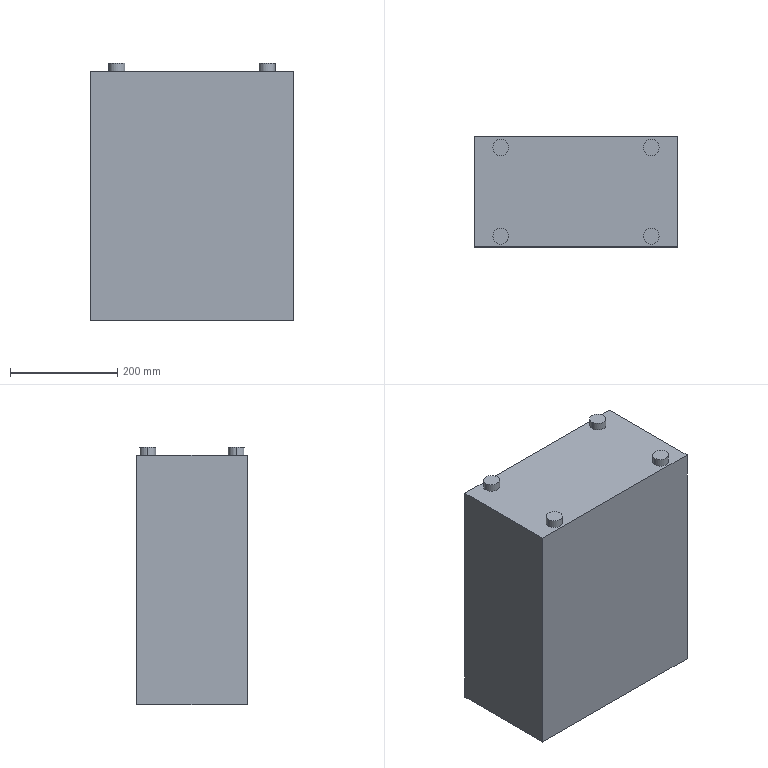Part | STEP file | PC | 1 solid | 18 faces | box 380 x 205 x 480 mm | volume 36265912 mm3 | plane 10 | cylinder 8 | commonest cylinder face diameters 30 x8
STEP:
#1=CARTESIAN_POINT('',(0.,0.,0.));
#2=DIRECTION('',(0.,0.,1.));
#3=DIRECTION('',(1.,0.,0.));
#4=AXIS2_PLACEMENT_3D('',#1,#2,#3);
#5=CARTESIAN_POINT('',(-125.,82.5,247.5));
#6=VERTEX_POINT('',#5);
#7=CARTESIAN_POINT('',(-155.,82.5,247.5));
#8=VERTEX_POINT('',#7);
#9=CARTESIAN_POINT('',(-140.,82.5,247.5));
#10=DIRECTION('',(0.,0.,1.));
#11=DIRECTION('',(-1.,0.,0.));
#12=AXIS2_PLACEMENT_3D('',#9,#10,#11);
#13=CIRCLE('',#12,15.);
#14=CARTESIAN_POINT('',(-140.,82.5,247.5));
#15=DIRECTION('',(0.,0.,-1.));
#16=DIRECTION('',(-1.,0.,0.));
#17=AXIS2_PLACEMENT_3D('',#14,#15,#16);
#18=CYLINDRICAL_SURFACE('',#17,15.);
#19=CARTESIAN_POINT('',(6.283,0.));
#20=DIRECTION('',(-1.,0.));
#21=VECTOR('',#20,1.);
#22=LINE('',#19,#21);
#23=(GEOMETRIC_REPRESENTATION_CONTEXT(2)PARAMETRIC_REPRESENTATION_CONTEXT()REPRESENTATION_CONTEXT('',''));
#24=DEFINITIONAL_REPRESENTATION('',(#22),#23);
#25=PCURVE('',#18,#24);
#26=CARTESIAN_POINT('',(-140.,82.5,247.5));
#27=DIRECTION('',(0.,0.,-1.));
#28=DIRECTION('',(-1.,0.,0.));
#29=AXIS2_PLACEMENT_3D('',#26,#27,#28);
#30=PLANE('',#29);
#31=CARTESIAN_POINT('',(15.,0.));
#32=CARTESIAN_POINT('',(15.,-25.981));
#33=CARTESIAN_POINT('',(-7.5,-12.99));
#34=CARTESIAN_POINT('',(-30.,0.));
#35=CARTESIAN_POINT('',(-7.5,12.99));
#36=CARTESIAN_POINT('',(15.,25.981));
#37=CARTESIAN_POINT('',(15.,0.));
#38=(BOUNDED_CURVE()B_SPLINE_CURVE(2,(#31,#32,#33,#34,#35,#36,#37),.UNSPECIFIED.,.T.,.F.)B_SPLINE_CURVE_WITH_KNOTS((1,2,2,2,2,1),(-2.094,0.,2.094,4.189,6.283,8.378),.UNSPECIFIED.)CURVE()GEOMETRIC_REPRESENTATION_ITEM()RATIONAL_B_SPLINE_CURVE((1.,0.5,1.,0.5,1.,0.5,1.))REPRESENTATION_ITEM(''));
#39=(GEOMETRIC_REPRESENTATION_CONTEXT(2)PARAMETRIC_REPRESENTATION_CONTEXT()REPRESENTATION_CONTEXT('',''));
#40=DEFINITIONAL_REPRESENTATION('',(#38),#39);
#41=PCURVE('',#30,#40);
#42=SURFACE_CURVE('',#13,(#25,#41),.PCURVE_S1.);
#43=EDGE_CURVE('',#6,#8,#42,.T.);
#44=ORIENTED_EDGE('',*,*,#43,.F.);
#45=CARTESIAN_POINT('',(-125.,82.5,232.5));
#46=VERTEX_POINT('',#45);
#47=CARTESIAN_POINT('',(-125.,82.5,247.5));
#48=DIRECTION('',(0.,0.,-1.));
#49=VECTOR('',#48,1.);
#50=LINE('',#47,#49);
#51=CARTESIAN_POINT('',(3.142,0.));
#52=DIRECTION('',(0.,1.));
#53=VECTOR('',#52,1.);
#54=LINE('',#51,#53);
#55=(GEOMETRIC_REPRESENTATION_CONTEXT(2)PARAMETRIC_REPRESENTATION_CONTEXT()REPRESENTATION_CONTEXT('',''));
#56=DEFINITIONAL_REPRESENTATION('',(#54),#55);
#57=PCURVE('',#18,#56);
#58=CARTESIAN_POINT('',(-140.,82.5,247.5));
#59=DIRECTION('',(0.,0.,-1.));
#60=DIRECTION('',(-1.,0.,0.));
#61=AXIS2_PLACEMENT_3D('',#58,#59,#60);
#62=CYLINDRICAL_SURFACE('',#61,15.);
#63=CARTESIAN_POINT('',(3.142,0.));
#64=DIRECTION('',(0.,1.));
#65=VECTOR('',#64,1.);
#66=LINE('',#63,#65);
#67=(GEOMETRIC_REPRESENTATION_CONTEXT(2)PARAMETRIC_REPRESENTATION_CONTEXT()REPRESENTATION_CONTEXT('',''));
#68=DEFINITIONAL_REPRESENTATION('',(#66),#67);
#69=PCURVE('',#62,#68);
#70=SURFACE_CURVE('',#50,(#57,#69),.PCURVE_S1.);
#71=EDGE_CURVE('',#6,#46,#70,.T.);
#72=ORIENTED_EDGE('',*,*,#71,.T.);
#73=CARTESIAN_POINT('',(-155.,82.5,232.5));
#74=VERTEX_POINT('',#73);
#75=CARTESIAN_POINT('',(-140.,82.5,232.5));
#76=DIRECTION('',(0.,0.,1.));
#77=DIRECTION('',(-1.,0.,0.));
#78=AXIS2_PLACEMENT_3D('',#75,#76,#77);
#79=CIRCLE('',#78,15.);
#80=CARTESIAN_POINT('',(6.283,15.));
#81=DIRECTION('',(-1.,0.));
#82=VECTOR('',#81,1.);
#83=LINE('',#80,#82);
#84=(GEOMETRIC_REPRESENTATION_CONTEXT(2)PARAMETRIC_REPRESENTATION_CONTEXT()REPRESENTATION_CONTEXT('',''));
#85=DEFINITIONAL_REPRESENTATION('',(#83),#84);
#86=PCURVE('',#18,#85);
#87=CARTESIAN_POINT('',(-190.,102.5,232.5));
#88=DIRECTION('',(0.,0.,-1.));
#89=DIRECTION('',(-1.,0.,0.));
#90=AXIS2_PLACEMENT_3D('',#87,#88,#89);
#91=PLANE('',#90);
#92=CARTESIAN_POINT('',(-35.,-20.));
#93=CARTESIAN_POINT('',(-35.,-45.981));
#94=CARTESIAN_POINT('',(-57.5,-32.99));
#95=CARTESIAN_POINT('',(-80.,-20.));
#96=CARTESIAN_POINT('',(-57.5,-7.01));
#97=CARTESIAN_POINT('',(-35.,5.981));
#98=CARTESIAN_POINT('',(-35.,-20.));
#99=(BOUNDED_CURVE()B_SPLINE_CURVE(2,(#92,#93,#94,#95,#96,#97,#98),.UNSPECIFIED.,.T.,.F.)B_SPLINE_CURVE_WITH_KNOTS((1,2,2,2,2,1),(-2.094,0.,2.094,4.189,6.283,8.378),.UNSPECIFIED.)CURVE()GEOMETRIC_REPRESENTATION_ITEM()RATIONAL_B_SPLINE_CURVE((1.,0.5,1.,0.5,1.,0.5,1.))REPRESENTATION_ITEM(''));
#100=(GEOMETRIC_REPRESENTATION_CONTEXT(2)PARAMETRIC_REPRESENTATION_CONTEXT()REPRESENTATION_CONTEXT('',''));
#101=DEFINITIONAL_REPRESENTATION('',(#99),#100);
#102=PCURVE('',#91,#101);
#103=SURFACE_CURVE('',#79,(#86,#102),.PCURVE_S1.);
#104=EDGE_CURVE('',#46,#74,#103,.T.);
#105=ORIENTED_EDGE('',*,*,#104,.T.);
#106=CARTESIAN_POINT('',(-155.,82.5,247.5));
#107=DIRECTION('',(0.,0.,-1.));
#108=VECTOR('',#107,1.);
#109=LINE('',#106,#108);
#110=CARTESIAN_POINT('',(0.,0.));
#111=DIRECTION('',(0.,1.));
#112=VECTOR('',#111,1.);
#113=LINE('',#110,#112);
#114=(GEOMETRIC_REPRESENTATION_CONTEXT(2)PARAMETRIC_REPRESENTATION_CONTEXT()REPRESENTATION_CONTEXT('',''));
#115=DEFINITIONAL_REPRESENTATION('',(#113),#114);
#116=PCURVE('',#18,#115);
#117=CARTESIAN_POINT('',(6.283,0.));
#118=DIRECTION('',(0.,1.));
#119=VECTOR('',#118,1.);
#120=LINE('',#117,#119);
#121=(GEOMETRIC_REPRESENTATION_CONTEXT(2)PARAMETRIC_REPRESENTATION_CONTEXT()REPRESENTATION_CONTEXT('',''));
#122=DEFINITIONAL_REPRESENTATION('',(#120),#121);
#123=PCURVE('',#62,#122);
#124=SURFACE_CURVE('',#109,(#116,#123),.PCURVE_S1.);
#125=EDGE_CURVE('',#8,#74,#124,.T.);
#126=ORIENTED_EDGE('',*,*,#125,.F.);
#127=EDGE_LOOP('',(#44,#72,#105,#126));
#128=FACE_BOUND('',#127,.T.);
#129=ADVANCED_FACE('',(#128),#18,.T.);
#130=CARTESIAN_POINT('',(-125.,-82.5,247.5));
#131=VERTEX_POINT('',#130);
#132=CARTESIAN_POINT('',(-155.,-82.5,247.5));
#133=VERTEX_POINT('',#132);
#134=CARTESIAN_POINT('',(-140.,-82.5,247.5));
#135=DIRECTION('',(0.,0.,1.));
#136=DIRECTION('',(1.,0.,0.));
#137=AXIS2_PLACEMENT_3D('',#134,#135,#136);
#138=CIRCLE('',#137,15.);
#139=CARTESIAN_POINT('',(-140.,-82.5,247.5));
#140=DIRECTION('',(0.,0.,-1.));
#141=DIRECTION('',(-1.,0.,0.));
#142=AXIS2_PLACEMENT_3D('',#139,#140,#141);
#143=CYLINDRICAL_SURFACE('',#142,15.);
#144=CARTESIAN_POINT('',(3.142,0.));
#145=DIRECTION('',(-1.,0.));
#146=VECTOR('',#145,1.);
#147=LINE('',#144,#146);
#148=(GEOMETRIC_REPRESENTATION_CONTEXT(2)PARAMETRIC_REPRESENTATION_CONTEXT()REPRESENTATION_CONTEXT('',''));
#149=DEFINITIONAL_REPRESENTATION('',(#147),#148);
#150=PCURVE('',#143,#149);
#151=CARTESIAN_POINT('',(-140.,-82.5,247.5));
#152=DIRECTION('',(0.,0.,1.));
#153=DIRECTION('',(1.,0.,0.));
#154=AXIS2_PLACEMENT_3D('',#151,#152,#153);
#155=PLANE('',#154);
#156=CARTESIAN_POINT('',(0.,0.));
#157=DIRECTION('',(1.,0.));
#158=AXIS2_PLACEMENT_2D('',#156,#157);
#159=CIRCLE('',#158,15.);
#160=(GEOMETRIC_REPRESENTATION_CONTEXT(2)PARAMETRIC_REPRESENTATION_CONTEXT()REPRESENTATION_CONTEXT('',''));
#161=DEFINITIONAL_REPRESENTATION('',(#159),#160);
#162=PCURVE('',#155,#161);
#163=SURFACE_CURVE('',#138,(#150,#162),.PCURVE_S1.);
#164=EDGE_CURVE('',#131,#133,#163,.T.);
#165=ORIENTED_EDGE('',*,*,#164,.F.);
#166=CARTESIAN_POINT('',(-125.,-82.5,232.5));
#167=VERTEX_POINT('',#166);
#168=CARTESIAN_POINT('',(-125.,-82.5,247.5));
#169=DIRECTION('',(0.,0.,-1.));
#170=VECTOR('',#169,1.);
#171=LINE('',#168,#170);
#172=CARTESIAN_POINT('',(3.142,0.));
#173=DIRECTION('',(0.,1.));
#174=VECTOR('',#173,1.);
#175=LINE('',#172,#174);
#176=(GEOMETRIC_REPRESENTATION_CONTEXT(2)PARAMETRIC_REPRESENTATION_CONTEXT()REPRESENTATION_CONTEXT('',''));
#177=DEFINITIONAL_REPRESENTATION('',(#175),#176);
#178=PCURVE('',#143,#177);
#179=CARTESIAN_POINT('',(-140.,-82.5,247.5));
#180=DIRECTION('',(0.,0.,-1.));
#181=DIRECTION('',(-1.,0.,0.));
#182=AXIS2_PLACEMENT_3D('',#179,#180,#181);
#183=CYLINDRICAL_SURFACE('',#182,15.);
#184=CARTESIAN_POINT('',(3.142,0.));
#185=DIRECTION('',(0.,1.));
#186=VECTOR('',#185,1.);
#187=LINE('',#184,#186);
#188=(GEOMETRIC_REPRESENTATION_CONTEXT(2)PARAMETRIC_REPRESENTATION_CONTEXT()REPRESENTATION_CONTEXT('',''));
#189=DEFINITIONAL_REPRESENTATION('',(#187),#188);
#190=PCURVE('',#183,#189);
#191=SURFACE_CURVE('',#171,(#178,#190),.PCURVE_S1.);
#192=EDGE_CURVE('',#131,#167,#191,.T.);
#193=ORIENTED_EDGE('',*,*,#192,.T.);
#194=CARTESIAN_POINT('',(-155.,-82.5,232.5));
#195=VERTEX_POINT('',#194);
#196=CARTESIAN_POINT('',(-140.,-82.5,232.5));
#197=DIRECTION('',(0.,0.,1.));
#198=DIRECTION('',(-1.,0.,0.));
#199=AXIS2_PLACEMENT_3D('',#196,#197,#198);
#200=CIRCLE('',#199,15.);
#201=CARTESIAN_POINT('',(6.283,15.));
#202=DIRECTION('',(-1.,0.));
#203=VECTOR('',#202,1.);
#204=LINE('',#201,#203);
#205=(GEOMETRIC_REPRESENTATION_CONTEXT(2)PARAMETRIC_REPRESENTATION_CONTEXT()REPRESENTATION_CONTEXT('',''));
#206=DEFINITIONAL_REPRESENTATION('',(#204),#205);
#207=PCURVE('',#143,#206);
#208=CARTESIAN_POINT('',(-35.,-185.));
#209=CARTESIAN_POINT('',(-35.,-210.981));
#210=CARTESIAN_POINT('',(-57.5,-197.99));
#211=CARTESIAN_POINT('',(-80.,-185.));
#212=CARTESIAN_POINT('',(-57.5,-172.01));
#213=CARTESIAN_POINT('',(-35.,-159.019));
#214=CARTESIAN_POINT('',(-35.,-185.));
#215=(BOUNDED_CURVE()B_SPLINE_CURVE(2,(#208,#209,#210,#211,#212,#213,#214),.UNSPECIFIED.,.T.,.F.)B_SPLINE_CURVE_WITH_KNOTS((1,2,2,2,2,1),(-2.094,0.,2.094,4.189,6.283,8.378),.UNSPECIFIED.)CURVE()GEOMETRIC_REPRESENTATION_ITEM()RATIONAL_B_SPLINE_CURVE((1.,0.5,1.,0.5,1.,0.5,1.))REPRESENTATION_ITEM(''));
#216=(GEOMETRIC_REPRESENTATION_CONTEXT(2)PARAMETRIC_REPRESENTATION_CONTEXT()REPRESENTATION_CONTEXT('',''));
#217=DEFINITIONAL_REPRESENTATION('',(#215),#216);
#218=PCURVE('',#91,#217);
#219=SURFACE_CURVE('',#200,(#207,#218),.PCURVE_S1.);
#220=EDGE_CURVE('',#167,#195,#219,.T.);
#221=ORIENTED_EDGE('',*,*,#220,.T.);
#222=CARTESIAN_POINT('',(-155.,-82.5,247.5));
#223=DIRECTION('',(0.,0.,-1.));
#224=VECTOR('',#223,1.);
#225=LINE('',#222,#224);
#226=CARTESIAN_POINT('',(0.,0.));
#227=DIRECTION('',(0.,1.));
#228=VECTOR('',#227,1.);
#229=LINE('',#226,#228);
#230=(GEOMETRIC_REPRESENTATION_CONTEXT(2)PARAMETRIC_REPRESENTATION_CONTEXT()REPRESENTATION_CONTEXT('',''));
#231=DEFINITIONAL_REPRESENTATION('',(#229),#230);
#232=PCURVE('',#143,#231);
#233=CARTESIAN_POINT('',(6.283,0.));
#234=DIRECTION('',(0.,1.));
#235=VECTOR('',#234,1.);
#236=LINE('',#233,#235);
#237=(GEOMETRIC_REPRESENTATION_CONTEXT(2)PARAMETRIC_REPRESENTATION_CONTEXT()REPRESENTATION_CONTEXT('',''));
#238=DEFINITIONAL_REPRESENTATION('',(#236),#237);
#239=PCURVE('',#183,#238);
#240=SURFACE_CURVE('',#225,(#232,#239),.PCURVE_S1.);
#241=EDGE_CURVE('',#133,#195,#240,.T.);
#242=ORIENTED_EDGE('',*,*,#241,.F.);
#243=EDGE_LOOP('',(#165,#193,#221,#242));
#244=FACE_BOUND('',#243,.T.);
#245=ADVANCED_FACE('',(#244),#143,.T.);
#246=CARTESIAN_POINT('',(155.,-82.5,247.5));
#247=VERTEX_POINT('',#246);
#248=CARTESIAN_POINT('',(125.,-82.5,247.5));
#249=VERTEX_POINT('',#248);
#250=CARTESIAN_POINT('',(140.,-82.5,247.5));
#251=DIRECTION('',(0.,0.,1.));
#252=DIRECTION('',(-1.,0.,0.));
#253=AXIS2_PLACEMENT_3D('',#250,#251,#252);
#254=CIRCLE('',#253,15.);
#255=CARTESIAN_POINT('',(140.,-82.5,247.5));
#256=DIRECTION('',(0.,0.,-1.));
#257=DIRECTION('',(-1.,0.,0.));
#258=AXIS2_PLACEMENT_3D('',#255,#256,#257);
#259=CYLINDRICAL_SURFACE('',#258,15.);
#260=CARTESIAN_POINT('',(6.283,0.));
#261=DIRECTION('',(-1.,0.));
#262=VECTOR('',#261,1.);
#263=LINE('',#260,#262);
#264=(GEOMETRIC_REPRESENTATION_CONTEXT(2)PARAMETRIC_REPRESENTATION_CONTEXT()REPRESENTATION_CONTEXT('',''));
#265=DEFINITIONAL_REPRESENTATION('',(#263),#264);
#266=PCURVE('',#259,#265);
#267=CARTESIAN_POINT('',(140.,-82.5,247.5));
#268=DIRECTION('',(0.,0.,-1.));
#269=DIRECTION('',(-1.,0.,0.));
#270=AXIS2_PLACEMENT_3D('',#267,#268,#269);
#271=PLANE('',#270);
#272=CARTESIAN_POINT('',(15.,0.));
#273=CARTESIAN_POINT('',(15.,-25.981));
#274=CARTESIAN_POINT('',(-7.5,-12.99));
#275=CARTESIAN_POINT('',(-30.,0.));
#276=CARTESIAN_POINT('',(-7.5,12.99));
#277=CARTESIAN_POINT('',(15.,25.981));
#278=CARTESIAN_POINT('',(15.,0.));
#279=(BOUNDED_CURVE()B_SPLINE_CURVE(2,(#272,#273,#274,#275,#276,#277,#278),.UNSPECIFIED.,.T.,.F.)B_SPLINE_CURVE_WITH_KNOTS((1,2,2,2,2,1),(-2.094,0.,2.094,4.189,6.283,8.378),.UNSPECIFIED.)CURVE()GEOMETRIC_REPRESENTATION_ITEM()RATIONAL_B_SPLINE_CURVE((1.,0.5,1.,0.5,1.,0.5,1.))REPRESENTATION_ITEM(''));
#280=(GEOMETRIC_REPRESENTATION_CONTEXT(2)PARAMETRIC_REPRESENTATION_CONTEXT()REPRESENTATION_CONTEXT('',''));
#281=DEFINITIONAL_REPRESENTATION('',(#279),#280);
#282=PCURVE('',#271,#281);
#283=SURFACE_CURVE('',#254,(#266,#282),.PCURVE_S1.);
#284=EDGE_CURVE('',#247,#249,#283,.T.);
#285=ORIENTED_EDGE('',*,*,#284,.F.);
#286=CARTESIAN_POINT('',(155.,-82.5,232.5));
#287=VERTEX_POINT('',#286);
#288=CARTESIAN_POINT('',(155.,-82.5,247.5));
#289=DIRECTION('',(0.,0.,-1.));
#290=VECTOR('',#289,1.);
#291=LINE('',#288,#290);
#292=CARTESIAN_POINT('',(3.142,0.));
#293=DIRECTION('',(0.,1.));
#294=VECTOR('',#293,1.);
#295=LINE('',#292,#294);
#296=(GEOMETRIC_REPRESENTATION_CONTEXT(2)PARAMETRIC_REPRESENTATION_CONTEXT()REPRESENTATION_CONTEXT('',''));
#297=DEFINITIONAL_REPRESENTATION('',(#295),#296);
#298=PCURVE('',#259,#297);
#299=CARTESIAN_POINT('',(140.,-82.5,247.5));
#300=DIRECTION('',(0.,0.,-1.));
#301=DIRECTION('',(-1.,0.,0.));
#302=AXIS2_PLACEMENT_3D('',#299,#300,#301);
#303=CYLINDRICAL_SURFACE('',#302,15.);
#304=CARTESIAN_POINT('',(3.142,0.));
#305=DIRECTION('',(0.,1.));
#306=VECTOR('',#305,1.);
#307=LINE('',#304,#306);
#308=(GEOMETRIC_REPRESENTATION_CONTEXT(2)PARAMETRIC_REPRESENTATION_CONTEXT()REPRESENTATION_CONTEXT('',''));
#309=DEFINITIONAL_REPRESENTATION('',(#307),#308);
#310=PCURVE('',#303,#309);
#311=SURFACE_CURVE('',#291,(#298,#310),.PCURVE_S1.);
#312=EDGE_CURVE('',#247,#287,#311,.T.);
#313=ORIENTED_EDGE('',*,*,#312,.T.);
#314=CARTESIAN_POINT('',(125.,-82.5,232.5));
#315=VERTEX_POINT('',#314);
#316=CARTESIAN_POINT('',(140.,-82.5,232.5));
#317=DIRECTION('',(0.,0.,1.));
#318=DIRECTION('',(-1.,0.,0.));
#319=AXIS2_PLACEMENT_3D('',#316,#317,#318);
#320=CIRCLE('',#319,15.);
#321=CARTESIAN_POINT('',(6.283,15.));
#322=DIRECTION('',(-1.,0.));
#323=VECTOR('',#322,1.);
#324=LINE('',#321,#323);
#325=(GEOMETRIC_REPRESENTATION_CONTEXT(2)PARAMETRIC_REPRESENTATION_CONTEXT()REPRESENTATION_CONTEXT('',''));
#326=DEFINITIONAL_REPRESENTATION('',(#324),#325);
#327=PCURVE('',#259,#326);
#328=CARTESIAN_POINT('',(-315.,-185.));
#329=CARTESIAN_POINT('',(-315.,-210.981));
#330=CARTESIAN_POINT('',(-337.5,-197.99));
#331=CARTESIAN_POINT('',(-360.,-185.));
#332=CARTESIAN_POINT('',(-337.5,-172.01));
#333=CARTESIAN_POINT('',(-315.,-159.019));
#334=CARTESIAN_POINT('',(-315.,-185.));
#335=(BOUNDED_CURVE()B_SPLINE_CURVE(2,(#328,#329,#330,#331,#332,#333,#334),.UNSPECIFIED.,.T.,.F.)B_SPLINE_CURVE_WITH_KNOTS((1,2,2,2,2,1),(-2.094,0.,2.094,4.189,6.283,8.378),.UNSPECIFIED.)CURVE()GEOMETRIC_REPRESENTATION_ITEM()RATIONAL_B_SPLINE_CURVE((1.,0.5,1.,0.5,1.,0.5,1.))REPRESENTATION_ITEM(''));
#336=(GEOMETRIC_REPRESENTATION_CONTEXT(2)PARAMETRIC_REPRESENTATION_CONTEXT()REPRESENTATION_CONTEXT('',''));
#337=DEFINITIONAL_REPRESENTATION('',(#335),#336);
#338=PCURVE('',#91,#337);
#339=SURFACE_CURVE('',#320,(#327,#338),.PCURVE_S1.);
#340=EDGE_CURVE('',#287,#315,#339,.T.);
#341=ORIENTED_EDGE('',*,*,#340,.T.);
#342=CARTESIAN_POINT('',(125.,-82.5,247.5));
#343=DIRECTION('',(0.,0.,-1.));
#344=VECTOR('',#343,1.);
#345=LINE('',#342,#344);
#346=CARTESIAN_POINT('',(0.,0.));
#347=DIRECTION('',(0.,1.));
#348=VECTOR('',#347,1.);
#349=LINE('',#346,#348);
#350=(GEOMETRIC_REPRESENTATION_CONTEXT(2)PARAMETRIC_REPRESENTATION_CONTEXT()REPRESENTATION_CONTEXT('',''));
#351=DEFINITIONAL_REPRESENTATION('',(#349),#350);
#352=PCURVE('',#259,#351);
#353=CARTESIAN_POINT('',(6.283,0.));
#354=DIRECTION('',(0.,1.));
#355=VECTOR('',#354,1.);
#356=LINE('',#353,#355);
#357=(GEOMETRIC_REPRESENTATION_CONTEXT(2)PARAMETRIC_REPRESENTATION_CONTEXT()REPRESENTATION_CONTEXT('',''));
#358=DEFINITIONAL_REPRESENTATION('',(#356),#357);
#359=PCURVE('',#303,#358);
#360=SURFACE_CURVE('',#345,(#352,#359),.PCURVE_S1.);
#361=EDGE_CURVE('',#249,#315,#360,.T.);
#362=ORIENTED_EDGE('',*,*,#361,.F.);
#363=EDGE_LOOP('',(#285,#313,#341,#362));
#364=FACE_BOUND('',#363,.T.);
#365=ADVANCED_FACE('',(#364),#259,.T.);
#366=CARTESIAN_POINT('',(155.,82.5,247.5));
#367=VERTEX_POINT('',#366);
#368=CARTESIAN_POINT('',(125.,82.5,247.5));
#369=VERTEX_POINT('',#368);
#370=CARTESIAN_POINT('',(140.,82.5,247.5));
#371=DIRECTION('',(0.,0.,1.));
#372=DIRECTION('',(1.,0.,0.));
#373=AXIS2_PLACEMENT_3D('',#370,#371,#372);
#374=CIRCLE('',#373,15.);
#375=CARTESIAN_POINT('',(140.,82.5,247.5));
#376=DIRECTION('',(0.,0.,-1.));
#377=DIRECTION('',(-1.,0.,0.));
#378=AXIS2_PLACEMENT_3D('',#375,#376,#377);
#379=CYLINDRICAL_SURFACE('',#378,15.);
#380=CARTESIAN_POINT('',(3.142,0.));
#381=DIRECTION('',(-1.,0.));
#382=VECTOR('',#381,1.);
#383=LINE('',#380,#382);
#384=(GEOMETRIC_REPRESENTATION_CONTEXT(2)PARAMETRIC_REPRESENTATION_CONTEXT()REPRESENTATION_CONTEXT('',''));
#385=DEFINITIONAL_REPRESENTATION('',(#383),#384);
#386=PCURVE('',#379,#385);
#387=CARTESIAN_POINT('',(140.,82.5,247.5));
#388=DIRECTION('',(0.,0.,1.));
#389=DIRECTION('',(1.,0.,0.));
#390=AXIS2_PLACEMENT_3D('',#387,#388,#389);
#391=PLANE('',#390);
#392=CARTESIAN_POINT('',(0.,0.));
#393=DIRECTION('',(1.,0.));
#394=AXIS2_PLACEMENT_2D('',#392,#393);
#395=CIRCLE('',#394,15.);
#396=(GEOMETRIC_REPRESENTATION_CONTEXT(2)PARAMETRIC_REPRESENTATION_CONTEXT()REPRESENTATION_CONTEXT('',''));
#397=DEFINITIONAL_REPRESENTATION('',(#395),#396);
#398=PCURVE('',#391,#397);
#399=SURFACE_CURVE('',#374,(#386,#398),.PCURVE_S1.);
#400=EDGE_CURVE('',#367,#369,#399,.T.);
#401=ORIENTED_EDGE('',*,*,#400,.F.);
#402=CARTESIAN_POINT('',(155.,82.5,232.5));
#403=VERTEX_POINT('',#402);
#404=CARTESIAN_POINT('',(155.,82.5,247.5));
#405=DIRECTION('',(0.,0.,-1.));
#406=VECTOR('',#405,1.);
#407=LINE('',#404,#406);
#408=CARTESIAN_POINT('',(3.142,0.));
#409=DIRECTION('',(0.,1.));
#410=VECTOR('',#409,1.);
#411=LINE('',#408,#410);
#412=(GEOMETRIC_REPRESENTATION_CONTEXT(2)PARAMETRIC_REPRESENTATION_CONTEXT()REPRESENTATION_CONTEXT('',''));
#413=DEFINITIONAL_REPRESENTATION('',(#411),#412);
#414=PCURVE('',#379,#413);
#415=CARTESIAN_POINT('',(140.,82.5,247.5));
#416=DIRECTION('',(0.,0.,-1.));
#417=DIRECTION('',(-1.,0.,0.));
#418=AXIS2_PLACEMENT_3D('',#415,#416,#417);
#419=CYLINDRICAL_SURFACE('',#418,15.);
#420=CARTESIAN_POINT('',(3.142,0.));
#421=DIRECTION('',(0.,1.));
#422=VECTOR('',#421,1.);
#423=LINE('',#420,#422);
#424=(GEOMETRIC_REPRESENTATION_CONTEXT(2)PARAMETRIC_REPRESENTATION_CONTEXT()REPRESENTATION_CONTEXT('',''));
#425=DEFINITIONAL_REPRESENTATION('',(#423),#424);
#426=PCURVE('',#419,#425);
#427=SURFACE_CURVE('',#407,(#414,#426),.PCURVE_S1.);
#428=EDGE_CURVE('',#367,#403,#427,.T.);
#429=ORIENTED_EDGE('',*,*,#428,.T.);
#430=CARTESIAN_POINT('',(125.,82.5,232.5));
#431=VERTEX_POINT('',#430);
#432=CARTESIAN_POINT('',(140.,82.5,232.5));
#433=DIRECTION('',(0.,0.,1.));
#434=DIRECTION('',(-1.,0.,0.));
#435=AXIS2_PLACEMENT_3D('',#432,#433,#434);
#436=CIRCLE('',#435,15.);
#437=CARTESIAN_POINT('',(6.283,15.));
#438=DIRECTION('',(-1.,0.));
#439=VECTOR('',#438,1.);
#440=LINE('',#437,#439);
#441=(GEOMETRIC_REPRESENTATION_CONTEXT(2)PARAMETRIC_REPRESENTATION_CONTEXT()REPRESENTATION_CONTEXT('',''));
#442=DEFINITIONAL_REPRESENTATION('',(#440),#441);
#443=PCURVE('',#379,#442);
#444=CARTESIAN_POINT('',(-315.,-20.));
#445=CARTESIAN_POINT('',(-315.,-45.981));
#446=CARTESIAN_POINT('',(-337.5,-32.99));
#447=CARTESIAN_POINT('',(-360.,-20.));
#448=CARTESIAN_POINT('',(-337.5,-7.01));
#449=CARTESIAN_POINT('',(-315.,5.981));
#450=CARTESIAN_POINT('',(-315.,-20.));
#451=(BOUNDED_CURVE()B_SPLINE_CURVE(2,(#444,#445,#446,#447,#448,#449,#450),.UNSPECIFIED.,.T.,.F.)B_SPLINE_CURVE_WITH_KNOTS((1,2,2,2,2,1),(-2.094,0.,2.094,4.189,6.283,8.378),.UNSPECIFIED.)CURVE()GEOMETRIC_REPRESENTATION_ITEM()RATIONAL_B_SPLINE_CURVE((1.,0.5,1.,0.5,1.,0.5,1.))REPRESENTATION_ITEM(''));
#452=(GEOMETRIC_REPRESENTATION_CONTEXT(2)PARAMETRIC_REPRESENTATION_CONTEXT()REPRESENTATION_CONTEXT('',''));
#453=DEFINITIONAL_REPRESENTATION('',(#451),#452);
#454=PCURVE('',#91,#453);
#455=SURFACE_CURVE('',#436,(#443,#454),.PCURVE_S1.);
#456=EDGE_CURVE('',#403,#431,#455,.T.);
#457=ORIENTED_EDGE('',*,*,#456,.T.);
#458=CARTESIAN_POINT('',(125.,82.5,247.5));
#459=DIRECTION('',(0.,0.,-1.));
#460=VECTOR('',#459,1.);
#461=LINE('',#458,#460);
#462=CARTESIAN_POINT('',(0.,0.));
#463=DIRECTION('',(0.,1.));
#464=VECTOR('',#463,1.);
#465=LINE('',#462,#464);
#466=(GEOMETRIC_REPRESENTATION_CONTEXT(2)PARAMETRIC_REPRESENTATION_CONTEXT()REPRESENTATION_CONTEXT('',''));
#467=DEFINITIONAL_REPRESENTATION('',(#465),#466);
#468=PCURVE('',#379,#467);
#469=CARTESIAN_POINT('',(6.283,0.));
#470=DIRECTION('',(0.,1.));
#471=VECTOR('',#470,1.);
#472=LINE('',#469,#471);
#473=(GEOMETRIC_REPRESENTATION_CONTEXT(2)PARAMETRIC_REPRESENTATION_CONTEXT()REPRESENTATION_CONTEXT('',''));
#474=DEFINITIONAL_REPRESENTATION('',(#472),#473);
#475=PCURVE('',#419,#474);
#476=SURFACE_CURVE('',#461,(#468,#475),.PCURVE_S1.);
#477=EDGE_CURVE('',#369,#431,#476,.T.);
#478=ORIENTED_EDGE('',*,*,#477,.F.);
#479=EDGE_LOOP('',(#401,#429,#457,#478));
#480=FACE_BOUND('',#479,.T.);
#481=ADVANCED_FACE('',(#480),#379,.T.);
#482=CARTESIAN_POINT('',(-190.,-102.5,-232.5));
#483=VERTEX_POINT('',#482);
#484=CARTESIAN_POINT('',(-190.,-102.5,232.5));
#485=VERTEX_POINT('',#484);
#486=CARTESIAN_POINT('',(-190.,-102.5,-232.5));
#487=DIRECTION('',(0.,0.,1.));
#488=VECTOR('',#487,1.);
#489=LINE('',#486,#488);
#490=CARTESIAN_POINT('',(-190.,102.5,-232.5));
#491=DIRECTION('',(1.,0.,0.));
#492=DIRECTION('',(0.,0.,-1.));
#493=AXIS2_PLACEMENT_3D('',#490,#491,#492);
#494=PLANE('',#493);
#495=CARTESIAN_POINT('',(0.,-205.));
#496=DIRECTION('',(-1.,0.));
#497=VECTOR('',#496,1.);
#498=LINE('',#495,#497);
#499=(GEOMETRIC_REPRESENTATION_CONTEXT(2)PARAMETRIC_REPRESENTATION_CONTEXT()REPRESENTATION_CONTEXT('',''));
#500=DEFINITIONAL_REPRESENTATION('',(#498),#499);
#501=PCURVE('',#494,#500);
#502=CARTESIAN_POINT('',(0.,-102.5,0.));
#503=DIRECTION('',(0.,1.,0.));
#504=DIRECTION('',(0.,0.,1.));
#505=AXIS2_PLACEMENT_3D('',#502,#503,#504);
#506=PLANE('',#505);
#507=CARTESIAN_POINT('',(-232.5,-190.));
#508=DIRECTION('',(1.,0.));
#509=VECTOR('',#508,1.);
#510=LINE('',#507,#509);
#511=(GEOMETRIC_REPRESENTATION_CONTEXT(2)PARAMETRIC_REPRESENTATION_CONTEXT()REPRESENTATION_CONTEXT('',''));
#512=DEFINITIONAL_REPRESENTATION('',(#510),#511);
#513=PCURVE('',#506,#512);
#514=SURFACE_CURVE('',#489,(#501,#513),.PCURVE_S1.);
#515=EDGE_CURVE('',#483,#485,#514,.T.);
#516=ORIENTED_EDGE('',*,*,#515,.T.);
#517=CARTESIAN_POINT('',(-190.,102.5,232.5));
#518=VERTEX_POINT('',#517);
#519=CARTESIAN_POINT('',(-190.,102.5,232.5));
#520=DIRECTION('',(0.,-1.,0.));
#521=VECTOR('',#520,1.);
#522=LINE('',#519,#521);
#523=CARTESIAN_POINT('',(-465.,0.));
#524=DIRECTION('',(0.,-1.));
#525=VECTOR('',#524,1.);
#526=LINE('',#523,#525);
#527=(GEOMETRIC_REPRESENTATION_CONTEXT(2)PARAMETRIC_REPRESENTATION_CONTEXT()REPRESENTATION_CONTEXT('',''));
#528=DEFINITIONAL_REPRESENTATION('',(#526),#527);
#529=PCURVE('',#494,#528);
#530=CARTESIAN_POINT('',(0.,0.));
#531=DIRECTION('',(0.,-1.));
#532=VECTOR('',#531,1.);
#533=LINE('',#530,#532);
#534=(GEOMETRIC_REPRESENTATION_CONTEXT(2)PARAMETRIC_REPRESENTATION_CONTEXT()REPRESENTATION_CONTEXT('',''));
#535=DEFINITIONAL_REPRESENTATION('',(#533),#534);
#536=PCURVE('',#91,#535);
#537=SURFACE_CURVE('',#522,(#529,#536),.PCURVE_S1.);
#538=EDGE_CURVE('',#518,#485,#537,.T.);
#539=ORIENTED_EDGE('',*,*,#538,.F.);
#540=CARTESIAN_POINT('',(-190.,102.5,-232.5));
#541=VERTEX_POINT('',#540);
#542=CARTESIAN_POINT('',(-190.,102.5,-232.5));
#543=DIRECTION('',(0.,0.,1.));
#544=VECTOR('',#543,1.);
#545=LINE('',#542,#544);
#546=CARTESIAN_POINT('',(0.,0.));
#547=DIRECTION('',(-1.,0.));
#548=VECTOR('',#547,1.);
#549=LINE('',#546,#548);
#550=(GEOMETRIC_REPRESENTATION_CONTEXT(2)PARAMETRIC_REPRESENTATION_CONTEXT()REPRESENTATION_CONTEXT('',''));
#551=DEFINITIONAL_REPRESENTATION('',(#549),#550);
#552=PCURVE('',#494,#551);
#553=CARTESIAN_POINT('',(0.,102.5,0.));
#554=DIRECTION('',(0.,1.,0.));
#555=DIRECTION('',(0.,0.,1.));
#556=AXIS2_PLACEMENT_3D('',#553,#554,#555);
#557=PLANE('',#556);
#558=CARTESIAN_POINT('',(-232.5,-190.));
#559=DIRECTION('',(1.,0.));
#560=VECTOR('',#559,1.);
#561=LINE('',#558,#560);
#562=(GEOMETRIC_REPRESENTATION_CONTEXT(2)PARAMETRIC_REPRESENTATION_CONTEXT()REPRESENTATION_CONTEXT('',''));
#563=DEFINITIONAL_REPRESENTATION('',(#561),#562);
#564=PCURVE('',#557,#563);
#565=SURFACE_CURVE('',#545,(#552,#564),.PCURVE_S1.);
#566=EDGE_CURVE('',#541,#518,#565,.T.);
#567=ORIENTED_EDGE('',*,*,#566,.F.);
#568=CARTESIAN_POINT('',(-190.,102.5,-232.5));
#569=DIRECTION('',(0.,-1.,0.));
#570=VECTOR('',#569,1.);
#571=LINE('',#568,#570);
#572=CARTESIAN_POINT('',(0.,0.));
#573=DIRECTION('',(0.,-1.));
#574=VECTOR('',#573,1.);
#575=LINE('',#572,#574);
#576=(GEOMETRIC_REPRESENTATION_CONTEXT(2)PARAMETRIC_REPRESENTATION_CONTEXT()REPRESENTATION_CONTEXT('',''));
#577=DEFINITIONAL_REPRESENTATION('',(#575),#576);
#578=PCURVE('',#494,#577);
#579=CARTESIAN_POINT('',(-190.,102.5,-232.5));
#580=DIRECTION('',(0.,0.,1.));
#581=DIRECTION('',(1.,0.,0.));
#582=AXIS2_PLACEMENT_3D('',#579,#580,#581);
#583=PLANE('',#582);
#584=CARTESIAN_POINT('',(0.,0.));
#585=DIRECTION('',(0.,-1.));
#586=VECTOR('',#585,1.);
#587=LINE('',#584,#586);
#588=(GEOMETRIC_REPRESENTATION_CONTEXT(2)PARAMETRIC_REPRESENTATION_CONTEXT()REPRESENTATION_CONTEXT('',''));
#589=DEFINITIONAL_REPRESENTATION('',(#587),#588);
#590=PCURVE('',#583,#589);
#591=SURFACE_CURVE('',#571,(#578,#590),.PCURVE_S1.);
#592=EDGE_CURVE('',#541,#483,#591,.T.);
#593=ORIENTED_EDGE('',*,*,#592,.T.);
#594=EDGE_LOOP('',(#516,#539,#567,#593));
#595=FACE_BOUND('',#594,.T.);
#596=ADVANCED_FACE('',(#595),#494,.F.);
#597=CARTESIAN_POINT('',(-140.,82.5,232.5));
#598=DIRECTION('',(0.,0.,1.));
#599=DIRECTION('',(-1.,0.,0.));
#600=AXIS2_PLACEMENT_3D('',#597,#598,#599);
#601=CIRCLE('',#600,15.);
#602=CARTESIAN_POINT('',(-35.,-20.));
#603=CARTESIAN_POINT('',(-35.,-45.981));
#604=CARTESIAN_POINT('',(-57.5,-32.99));
#605=CARTESIAN_POINT('',(-80.,-20.));
#606=CARTESIAN_POINT('',(-57.5,-7.01));
#607=CARTESIAN_POINT('',(-35.,5.981));
#608=CARTESIAN_POINT('',(-35.,-20.));
#609=(BOUNDED_CURVE()B_SPLINE_CURVE(2,(#602,#603,#604,#605,#606,#607,#608),.UNSPECIFIED.,.T.,.F.)B_SPLINE_CURVE_WITH_KNOTS((1,2,2,2,2,1),(-2.094,0.,2.094,4.189,6.283,8.378),.UNSPECIFIED.)CURVE()GEOMETRIC_REPRESENTATION_ITEM()RATIONAL_B_SPLINE_CURVE((1.,0.5,1.,0.5,1.,0.5,1.))REPRESENTATION_ITEM(''));
#610=(GEOMETRIC_REPRESENTATION_CONTEXT(2)PARAMETRIC_REPRESENTATION_CONTEXT()REPRESENTATION_CONTEXT('',''));
#611=DEFINITIONAL_REPRESENTATION('',(#609),#610);
#612=PCURVE('',#91,#611);
#613=CARTESIAN_POINT('',(6.283,15.));
#614=DIRECTION('',(-1.,0.));
#615=VECTOR('',#614,1.);
#616=LINE('',#613,#615);
#617=(GEOMETRIC_REPRESENTATION_CONTEXT(2)PARAMETRIC_REPRESENTATION_CONTEXT()REPRESENTATION_CONTEXT('',''));
#618=DEFINITIONAL_REPRESENTATION('',(#616),#617);
#619=PCURVE('',#62,#618);
#620=SURFACE_CURVE('',#601,(#612,#619),.PCURVE_S1.);
#621=EDGE_CURVE('',#74,#46,#620,.T.);
#622=ORIENTED_EDGE('',*,*,#621,.F.);
#623=ORIENTED_EDGE('',*,*,#104,.F.);
#624=EDGE_LOOP('',(#622,#623));
#625=FACE_BOUND('',#624,.T.);
#626=CARTESIAN_POINT('',(-140.,-82.5,232.5));
#627=DIRECTION('',(0.,0.,1.));
#628=DIRECTION('',(-1.,0.,0.));
#629=AXIS2_PLACEMENT_3D('',#626,#627,#628);
#630=CIRCLE('',#629,15.);
#631=CARTESIAN_POINT('',(-35.,-185.));
#632=CARTESIAN_POINT('',(-35.,-210.981));
#633=CARTESIAN_POINT('',(-57.5,-197.99));
#634=CARTESIAN_POINT('',(-80.,-185.));
#635=CARTESIAN_POINT('',(-57.5,-172.01));
#636=CARTESIAN_POINT('',(-35.,-159.019));
#637=CARTESIAN_POINT('',(-35.,-185.));
#638=(BOUNDED_CURVE()B_SPLINE_CURVE(2,(#631,#632,#633,#634,#635,#636,#637),.UNSPECIFIED.,.T.,.F.)B_SPLINE_CURVE_WITH_KNOTS((1,2,2,2,2,1),(-2.094,0.,2.094,4.189,6.283,8.378),.UNSPECIFIED.)CURVE()GEOMETRIC_REPRESENTATION_ITEM()RATIONAL_B_SPLINE_CURVE((1.,0.5,1.,0.5,1.,0.5,1.))REPRESENTATION_ITEM(''));
#639=(GEOMETRIC_REPRESENTATION_CONTEXT(2)PARAMETRIC_REPRESENTATION_CONTEXT()REPRESENTATION_CONTEXT('',''));
#640=DEFINITIONAL_REPRESENTATION('',(#638),#639);
#641=PCURVE('',#91,#640);
#642=CARTESIAN_POINT('',(6.283,15.));
#643=DIRECTION('',(-1.,0.));
#644=VECTOR('',#643,1.);
#645=LINE('',#642,#644);
#646=(GEOMETRIC_REPRESENTATION_CONTEXT(2)PARAMETRIC_REPRESENTATION_CONTEXT()REPRESENTATION_CONTEXT('',''));
#647=DEFINITIONAL_REPRESENTATION('',(#645),#646);
#648=PCURVE('',#183,#647);
#649=SURFACE_CURVE('',#630,(#641,#648),.PCURVE_S1.);
#650=EDGE_CURVE('',#195,#167,#649,.T.);
#651=ORIENTED_EDGE('',*,*,#650,.F.);
#652=ORIENTED_EDGE('',*,*,#220,.F.);
#653=EDGE_LOOP('',(#651,#652));
#654=FACE_BOUND('',#653,.T.);
#655=CARTESIAN_POINT('',(140.,-82.5,232.5));
#656=DIRECTION('',(0.,0.,1.));
#657=DIRECTION('',(-1.,0.,0.));
#658=AXIS2_PLACEMENT_3D('',#655,#656,#657);
#659=CIRCLE('',#658,15.);
#660=CARTESIAN_POINT('',(-315.,-185.));
#661=CARTESIAN_POINT('',(-315.,-210.981));
#662=CARTESIAN_POINT('',(-337.5,-197.99));
#663=CARTESIAN_POINT('',(-360.,-185.));
#664=CARTESIAN_POINT('',(-337.5,-172.01));
#665=CARTESIAN_POINT('',(-315.,-159.019));
#666=CARTESIAN_POINT('',(-315.,-185.));
#667=(BOUNDED_CURVE()B_SPLINE_CURVE(2,(#660,#661,#662,#663,#664,#665,#666),.UNSPECIFIED.,.T.,.F.)B_SPLINE_CURVE_WITH_KNOTS((1,2,2,2,2,1),(-2.094,0.,2.094,4.189,6.283,8.378),.UNSPECIFIED.)CURVE()GEOMETRIC_REPRESENTATION_ITEM()RATIONAL_B_SPLINE_CURVE((1.,0.5,1.,0.5,1.,0.5,1.))REPRESENTATION_ITEM(''));
#668=(GEOMETRIC_REPRESENTATION_CONTEXT(2)PARAMETRIC_REPRESENTATION_CONTEXT()REPRESENTATION_CONTEXT('',''));
#669=DEFINITIONAL_REPRESENTATION('',(#667),#668);
#670=PCURVE('',#91,#669);
#671=CARTESIAN_POINT('',(6.283,15.));
#672=DIRECTION('',(-1.,0.));
#673=VECTOR('',#672,1.);
#674=LINE('',#671,#673);
#675=(GEOMETRIC_REPRESENTATION_CONTEXT(2)PARAMETRIC_REPRESENTATION_CONTEXT()REPRESENTATION_CONTEXT('',''));
#676=DEFINITIONAL_REPRESENTATION('',(#674),#675);
#677=PCURVE('',#303,#676);
#678=SURFACE_CURVE('',#659,(#670,#677),.PCURVE_S1.);
#679=EDGE_CURVE('',#315,#287,#678,.T.);
#680=ORIENTED_EDGE('',*,*,#679,.F.);
#681=ORIENTED_EDGE('',*,*,#340,.F.);
#682=EDGE_LOOP('',(#680,#681));
#683=FACE_BOUND('',#682,.T.);
#684=CARTESIAN_POINT('',(140.,82.5,232.5));
#685=DIRECTION('',(0.,0.,1.));
#686=DIRECTION('',(-1.,0.,0.));
#687=AXIS2_PLACEMENT_3D('',#684,#685,#686);
#688=CIRCLE('',#687,15.);
#689=CARTESIAN_POINT('',(-315.,-20.));
#690=CARTESIAN_POINT('',(-315.,-45.981));
#691=CARTESIAN_POINT('',(-337.5,-32.99));
#692=CARTESIAN_POINT('',(-360.,-20.));
#693=CARTESIAN_POINT('',(-337.5,-7.01));
#694=CARTESIAN_POINT('',(-315.,5.981));
#695=CARTESIAN_POINT('',(-315.,-20.));
#696=(BOUNDED_CURVE()B_SPLINE_CURVE(2,(#689,#690,#691,#692,#693,#694,#695),.UNSPECIFIED.,.T.,.F.)B_SPLINE_CURVE_WITH_KNOTS((1,2,2,2,2,1),(-2.094,0.,2.094,4.189,6.283,8.378),.UNSPECIFIED.)CURVE()GEOMETRIC_REPRESENTATION_ITEM()RATIONAL_B_SPLINE_CURVE((1.,0.5,1.,0.5,1.,0.5,1.))REPRESENTATION_ITEM(''));
#697=(GEOMETRIC_REPRESENTATION_CONTEXT(2)PARAMETRIC_REPRESENTATION_CONTEXT()REPRESENTATION_CONTEXT('',''));
#698=DEFINITIONAL_REPRESENTATION('',(#696),#697);
#699=PCURVE('',#91,#698);
#700=CARTESIAN_POINT('',(6.283,15.));
#701=DIRECTION('',(-1.,0.));
#702=VECTOR('',#701,1.);
#703=LINE('',#700,#702);
#704=(GEOMETRIC_REPRESENTATION_CONTEXT(2)PARAMETRIC_REPRESENTATION_CONTEXT()REPRESENTATION_CONTEXT('',''));
#705=DEFINITIONAL_REPRESENTATION('',(#703),#704);
#706=PCURVE('',#419,#705);
#707=SURFACE_CURVE('',#688,(#699,#706),.PCURVE_S1.);
#708=EDGE_CURVE('',#431,#403,#707,.T.);
#709=ORIENTED_EDGE('',*,*,#708,.F.);
#710=ORIENTED_EDGE('',*,*,#456,.F.);
#711=EDGE_LOOP('',(#709,#710));
#712=FACE_BOUND('',#711,.T.);
#713=CARTESIAN_POINT('',(190.,-102.5,232.5));
#714=VERTEX_POINT('',#713);
#715=CARTESIAN_POINT('',(-190.,-102.5,232.5));
#716=DIRECTION('',(1.,0.,0.));
#717=VECTOR('',#716,1.);
#718=LINE('',#715,#717);
#719=CARTESIAN_POINT('',(0.,-205.));
#720=DIRECTION('',(-1.,0.));
#721=VECTOR('',#720,1.);
#722=LINE('',#719,#721);
#723=(GEOMETRIC_REPRESENTATION_CONTEXT(2)PARAMETRIC_REPRESENTATION_CONTEXT()REPRESENTATION_CONTEXT('',''));
#724=DEFINITIONAL_REPRESENTATION('',(#722),#723);
#725=PCURVE('',#91,#724);
#726=CARTESIAN_POINT('',(232.5,-190.));
#727=DIRECTION('',(0.,1.));
#728=VECTOR('',#727,1.);
#729=LINE('',#726,#728);
#730=(GEOMETRIC_REPRESENTATION_CONTEXT(2)PARAMETRIC_REPRESENTATION_CONTEXT()REPRESENTATION_CONTEXT('',''));
#731=DEFINITIONAL_REPRESENTATION('',(#729),#730);
#732=PCURVE('',#506,#731);
#733=SURFACE_CURVE('',#718,(#725,#732),.PCURVE_S1.);
#734=EDGE_CURVE('',#485,#714,#733,.T.);
#735=ORIENTED_EDGE('',*,*,#734,.T.);
#736=CARTESIAN_POINT('',(190.,102.5,232.5));
#737=VERTEX_POINT('',#736);
#738=CARTESIAN_POINT('',(190.,102.5,232.5));
#739=DIRECTION('',(0.,-1.,0.));
#740=VECTOR('',#739,1.);
#741=LINE('',#738,#740);
#742=CARTESIAN_POINT('',(-380.,0.));
#743=DIRECTION('',(0.,-1.));
#744=VECTOR('',#743,1.);
#745=LINE('',#742,#744);
#746=(GEOMETRIC_REPRESENTATION_CONTEXT(2)PARAMETRIC_REPRESENTATION_CONTEXT()REPRESENTATION_CONTEXT('',''));
#747=DEFINITIONAL_REPRESENTATION('',(#745),#746);
#748=PCURVE('',#91,#747);
#749=CARTESIAN_POINT('',(190.,102.5,-232.5));
#750=DIRECTION('',(-1.,0.,0.));
#751=DIRECTION('',(0.,0.,1.));
#752=AXIS2_PLACEMENT_3D('',#749,#750,#751);
#753=PLANE('',#752);
#754=CARTESIAN_POINT('',(465.,0.));
#755=DIRECTION('',(0.,-1.));
#756=VECTOR('',#755,1.);
#757=LINE('',#754,#756);
#758=(GEOMETRIC_REPRESENTATION_CONTEXT(2)PARAMETRIC_REPRESENTATION_CONTEXT()REPRESENTATION_CONTEXT('',''));
#759=DEFINITIONAL_REPRESENTATION('',(#757),#758);
#760=PCURVE('',#753,#759);
#761=SURFACE_CURVE('',#741,(#748,#760),.PCURVE_S1.);
#762=EDGE_CURVE('',#737,#714,#761,.T.);
#763=ORIENTED_EDGE('',*,*,#762,.F.);
#764=CARTESIAN_POINT('',(-190.,102.5,232.5));
#765=DIRECTION('',(1.,0.,0.));
#766=VECTOR('',#765,1.);
#767=LINE('',#764,#766);
#768=CARTESIAN_POINT('',(0.,0.));
#769=DIRECTION('',(-1.,0.));
#770=VECTOR('',#769,1.);
#771=LINE('',#768,#770);
#772=(GEOMETRIC_REPRESENTATION_CONTEXT(2)PARAMETRIC_REPRESENTATION_CONTEXT()REPRESENTATION_CONTEXT('',''));
#773=DEFINITIONAL_REPRESENTATION('',(#771),#772);
#774=PCURVE('',#91,#773);
#775=CARTESIAN_POINT('',(232.5,-190.));
#776=DIRECTION('',(0.,1.));
#777=VECTOR('',#776,1.);
#778=LINE('',#775,#777);
#779=(GEOMETRIC_REPRESENTATION_CONTEXT(2)PARAMETRIC_REPRESENTATION_CONTEXT()REPRESENTATION_CONTEXT('',''));
#780=DEFINITIONAL_REPRESENTATION('',(#778),#779);
#781=PCURVE('',#557,#780);
#782=SURFACE_CURVE('',#767,(#774,#781),.PCURVE_S1.);
#783=EDGE_CURVE('',#518,#737,#782,.T.);
#784=ORIENTED_EDGE('',*,*,#783,.F.);
#785=ORIENTED_EDGE('',*,*,#538,.T.);
#786=EDGE_LOOP('',(#735,#763,#784,#785));
#787=FACE_BOUND('',#786,.T.);
#788=ADVANCED_FACE('',(#625,#654,#683,#712,#787),#91,.F.);
#789=CARTESIAN_POINT('',(190.,-102.5,-232.5));
#790=VERTEX_POINT('',#789);
#791=CARTESIAN_POINT('',(190.,-102.5,-232.5));
#792=DIRECTION('',(0.,0.,-1.));
#793=VECTOR('',#792,1.);
#794=LINE('',#791,#793);
#795=CARTESIAN_POINT('',(0.,-205.));
#796=DIRECTION('',(-1.,0.));
#797=VECTOR('',#796,1.);
#798=LINE('',#795,#797);
#799=(GEOMETRIC_REPRESENTATION_CONTEXT(2)PARAMETRIC_REPRESENTATION_CONTEXT()REPRESENTATION_CONTEXT('',''));
#800=DEFINITIONAL_REPRESENTATION('',(#798),#799);
#801=PCURVE('',#753,#800);
#802=CARTESIAN_POINT('',(-232.5,190.));
#803=DIRECTION('',(-1.,0.));
#804=VECTOR('',#803,1.);
#805=LINE('',#802,#804);
#806=(GEOMETRIC_REPRESENTATION_CONTEXT(2)PARAMETRIC_REPRESENTATION_CONTEXT()REPRESENTATION_CONTEXT('',''));
#807=DEFINITIONAL_REPRESENTATION('',(#805),#806);
#808=PCURVE('',#506,#807);
#809=SURFACE_CURVE('',#794,(#801,#808),.PCURVE_S1.);
#810=EDGE_CURVE('',#714,#790,#809,.T.);
#811=ORIENTED_EDGE('',*,*,#810,.T.);
#812=CARTESIAN_POINT('',(190.,102.5,-232.5));
#813=VERTEX_POINT('',#812);
#814=CARTESIAN_POINT('',(190.,102.5,-232.5));
#815=DIRECTION('',(0.,-1.,0.));
#816=VECTOR('',#815,1.);
#817=LINE('',#814,#816);
#818=CARTESIAN_POINT('',(0.,0.));
#819=DIRECTION('',(0.,-1.));
#820=VECTOR('',#819,1.);
#821=LINE('',#818,#820);
#822=(GEOMETRIC_REPRESENTATION_CONTEXT(2)PARAMETRIC_REPRESENTATION_CONTEXT()REPRESENTATION_CONTEXT('',''));
#823=DEFINITIONAL_REPRESENTATION('',(#821),#822);
#824=PCURVE('',#753,#823);
#825=CARTESIAN_POINT('',(380.,0.));
#826=DIRECTION('',(0.,-1.));
#827=VECTOR('',#826,1.);
#828=LINE('',#825,#827);
#829=(GEOMETRIC_REPRESENTATION_CONTEXT(2)PARAMETRIC_REPRESENTATION_CONTEXT()REPRESENTATION_CONTEXT('',''));
#830=DEFINITIONAL_REPRESENTATION('',(#828),#829);
#831=PCURVE('',#583,#830);
#832=SURFACE_CURVE('',#817,(#824,#831),.PCURVE_S1.);
#833=EDGE_CURVE('',#813,#790,#832,.T.);
#834=ORIENTED_EDGE('',*,*,#833,.F.);
#835=CARTESIAN_POINT('',(190.,102.5,-232.5));
#836=DIRECTION('',(0.,0.,-1.));
#837=VECTOR('',#836,1.);
#838=LINE('',#835,#837);
#839=CARTESIAN_POINT('',(0.,0.));
#840=DIRECTION('',(-1.,0.));
#841=VECTOR('',#840,1.);
#842=LINE('',#839,#841);
#843=(GEOMETRIC_REPRESENTATION_CONTEXT(2)PARAMETRIC_REPRESENTATION_CONTEXT()REPRESENTATION_CONTEXT('',''));
#844=DEFINITIONAL_REPRESENTATION('',(#842),#843);
#845=PCURVE('',#753,#844);
#846=CARTESIAN_POINT('',(-232.5,190.));
#847=DIRECTION('',(-1.,0.));
#848=VECTOR('',#847,1.);
#849=LINE('',#846,#848);
#850=(GEOMETRIC_REPRESENTATION_CONTEXT(2)PARAMETRIC_REPRESENTATION_CONTEXT()REPRESENTATION_CONTEXT('',''));
#851=DEFINITIONAL_REPRESENTATION('',(#849),#850);
#852=PCURVE('',#557,#851);
#853=SURFACE_CURVE('',#838,(#845,#852),.PCURVE_S1.);
#854=EDGE_CURVE('',#737,#813,#853,.T.);
#855=ORIENTED_EDGE('',*,*,#854,.F.);
#856=ORIENTED_EDGE('',*,*,#762,.T.);
#857=EDGE_LOOP('',(#811,#834,#855,#856));
#858=FACE_BOUND('',#857,.T.);
#859=ADVANCED_FACE('',(#858),#753,.F.);
#860=CARTESIAN_POINT('',(-190.,-102.5,-232.5));
#861=DIRECTION('',(-1.,0.,0.));
#862=VECTOR('',#861,1.);
#863=LINE('',#860,#862);
#864=CARTESIAN_POINT('',(0.,-205.));
#865=DIRECTION('',(-1.,0.));
#866=VECTOR('',#865,1.);
#867=LINE('',#864,#866);
#868=(GEOMETRIC_REPRESENTATION_CONTEXT(2)PARAMETRIC_REPRESENTATION_CONTEXT()REPRESENTATION_CONTEXT('',''));
#869=DEFINITIONAL_REPRESENTATION('',(#867),#868);
#870=PCURVE('',#583,#869);
#871=CARTESIAN_POINT('',(-232.5,-190.));
#872=DIRECTION('',(0.,-1.));
#873=VECTOR('',#872,1.);
#874=LINE('',#871,#873);
#875=(GEOMETRIC_REPRESENTATION_CONTEXT(2)PARAMETRIC_REPRESENTATION_CONTEXT()REPRESENTATION_CONTEXT('',''));
#876=DEFINITIONAL_REPRESENTATION('',(#874),#875);
#877=PCURVE('',#506,#876);
#878=SURFACE_CURVE('',#863,(#870,#877),.PCURVE_S1.);
#879=EDGE_CURVE('',#790,#483,#878,.T.);
#880=ORIENTED_EDGE('',*,*,#879,.T.);
#881=ORIENTED_EDGE('',*,*,#592,.F.);
#882=CARTESIAN_POINT('',(-190.,102.5,-232.5));
#883=DIRECTION('',(-1.,0.,0.));
#884=VECTOR('',#883,1.);
#885=LINE('',#882,#884);
#886=CARTESIAN_POINT('',(0.,0.));
#887=DIRECTION('',(-1.,0.));
#888=VECTOR('',#887,1.);
#889=LINE('',#886,#888);
#890=(GEOMETRIC_REPRESENTATION_CONTEXT(2)PARAMETRIC_REPRESENTATION_CONTEXT()REPRESENTATION_CONTEXT('',''));
#891=DEFINITIONAL_REPRESENTATION('',(#889),#890);
#892=PCURVE('',#583,#891);
#893=CARTESIAN_POINT('',(-232.5,-190.));
#894=DIRECTION('',(0.,-1.));
#895=VECTOR('',#894,1.);
#896=LINE('',#893,#895);
#897=(GEOMETRIC_REPRESENTATION_CONTEXT(2)PARAMETRIC_REPRESENTATION_CONTEXT()REPRESENTATION_CONTEXT('',''));
#898=DEFINITIONAL_REPRESENTATION('',(#896),#897);
#899=PCURVE('',#557,#898);
#900=SURFACE_CURVE('',#885,(#892,#899),.PCURVE_S1.);
#901=EDGE_CURVE('',#813,#541,#900,.T.);
#902=ORIENTED_EDGE('',*,*,#901,.F.);
#903=ORIENTED_EDGE('',*,*,#833,.T.);
#904=EDGE_LOOP('',(#880,#881,#902,#903));
#905=FACE_BOUND('',#904,.T.);
#906=ADVANCED_FACE('',(#905),#583,.F.);
#907=ORIENTED_EDGE('',*,*,#566,.T.);
#908=ORIENTED_EDGE('',*,*,#783,.T.);
#909=ORIENTED_EDGE('',*,*,#854,.T.);
#910=ORIENTED_EDGE('',*,*,#901,.T.);
#911=EDGE_LOOP('',(#907,#908,#909,#910));
#912=FACE_BOUND('',#911,.T.);
#913=ADVANCED_FACE('',(#912),#557,.T.);
#914=ORIENTED_EDGE('',*,*,#515,.F.);
#915=ORIENTED_EDGE('',*,*,#879,.F.);
#916=ORIENTED_EDGE('',*,*,#810,.F.);
#917=ORIENTED_EDGE('',*,*,#734,.F.);
#918=EDGE_LOOP('',(#914,#915,#916,#917));
#919=FACE_BOUND('',#918,.T.);
#920=ADVANCED_FACE('',(#919),#506,.F.);
#921=ORIENTED_EDGE('',*,*,#428,.F.);
#922=CARTESIAN_POINT('',(140.,82.5,247.5));
#923=DIRECTION('',(0.,0.,1.));
#924=DIRECTION('',(1.,0.,0.));
#925=AXIS2_PLACEMENT_3D('',#922,#923,#924);
#926=CIRCLE('',#925,15.);
#927=CARTESIAN_POINT('',(9.425,0.));
#928=DIRECTION('',(-1.,0.));
#929=VECTOR('',#928,1.);
#930=LINE('',#927,#929);
#931=(GEOMETRIC_REPRESENTATION_CONTEXT(2)PARAMETRIC_REPRESENTATION_CONTEXT()REPRESENTATION_CONTEXT('',''));
#932=DEFINITIONAL_REPRESENTATION('',(#930),#931);
#933=PCURVE('',#419,#932);
#934=CARTESIAN_POINT('',(0.,0.));
#935=DIRECTION('',(1.,0.));
#936=AXIS2_PLACEMENT_2D('',#934,#935);
#937=CIRCLE('',#936,15.);
#938=(GEOMETRIC_REPRESENTATION_CONTEXT(2)PARAMETRIC_REPRESENTATION_CONTEXT()REPRESENTATION_CONTEXT('',''));
#939=DEFINITIONAL_REPRESENTATION('',(#937),#938);
#940=PCURVE('',#391,#939);
#941=SURFACE_CURVE('',#926,(#933,#940),.PCURVE_S1.);
#942=EDGE_CURVE('',#369,#367,#941,.T.);
#943=ORIENTED_EDGE('',*,*,#942,.F.);
#944=ORIENTED_EDGE('',*,*,#477,.T.);
#945=ORIENTED_EDGE('',*,*,#708,.T.);
#946=EDGE_LOOP('',(#921,#943,#944,#945));
#947=FACE_BOUND('',#946,.T.);
#948=ADVANCED_FACE('',(#947),#419,.T.);
#949=ORIENTED_EDGE('',*,*,#942,.T.);
#950=ORIENTED_EDGE('',*,*,#400,.T.);
#951=EDGE_LOOP('',(#949,#950));
#952=FACE_BOUND('',#951,.T.);
#953=ADVANCED_FACE('',(#952),#391,.T.);
#954=ORIENTED_EDGE('',*,*,#312,.F.);
#955=CARTESIAN_POINT('',(140.,-82.5,247.5));
#956=DIRECTION('',(0.,0.,1.));
#957=DIRECTION('',(-1.,0.,0.));
#958=AXIS2_PLACEMENT_3D('',#955,#956,#957);
#959=CIRCLE('',#958,15.);
#960=CARTESIAN_POINT('',(6.283,0.));
#961=DIRECTION('',(-1.,0.));
#962=VECTOR('',#961,1.);
#963=LINE('',#960,#962);
#964=(GEOMETRIC_REPRESENTATION_CONTEXT(2)PARAMETRIC_REPRESENTATION_CONTEXT()REPRESENTATION_CONTEXT('',''));
#965=DEFINITIONAL_REPRESENTATION('',(#963),#964);
#966=PCURVE('',#303,#965);
#967=CARTESIAN_POINT('',(15.,0.));
#968=CARTESIAN_POINT('',(15.,-25.981));
#969=CARTESIAN_POINT('',(-7.5,-12.99));
#970=CARTESIAN_POINT('',(-30.,0.));
#971=CARTESIAN_POINT('',(-7.5,12.99));
#972=CARTESIAN_POINT('',(15.,25.981));
#973=CARTESIAN_POINT('',(15.,0.));
#974=(BOUNDED_CURVE()B_SPLINE_CURVE(2,(#967,#968,#969,#970,#971,#972,#973),.UNSPECIFIED.,.T.,.F.)B_SPLINE_CURVE_WITH_KNOTS((1,2,2,2,2,1),(-2.094,0.,2.094,4.189,6.283,8.378),.UNSPECIFIED.)CURVE()GEOMETRIC_REPRESENTATION_ITEM()RATIONAL_B_SPLINE_CURVE((1.,0.5,1.,0.5,1.,0.5,1.))REPRESENTATION_ITEM(''));
#975=(GEOMETRIC_REPRESENTATION_CONTEXT(2)PARAMETRIC_REPRESENTATION_CONTEXT()REPRESENTATION_CONTEXT('',''));
#976=DEFINITIONAL_REPRESENTATION('',(#974),#975);
#977=PCURVE('',#271,#976);
#978=SURFACE_CURVE('',#959,(#966,#977),.PCURVE_S1.);
#979=EDGE_CURVE('',#249,#247,#978,.T.);
#980=ORIENTED_EDGE('',*,*,#979,.F.);
#981=ORIENTED_EDGE('',*,*,#361,.T.);
#982=ORIENTED_EDGE('',*,*,#679,.T.);
#983=EDGE_LOOP('',(#954,#980,#981,#982));
#984=FACE_BOUND('',#983,.T.);
#985=ADVANCED_FACE('',(#984),#303,.T.);
#986=ORIENTED_EDGE('',*,*,#979,.T.);
#987=ORIENTED_EDGE('',*,*,#284,.T.);
#988=EDGE_LOOP('',(#986,#987));
#989=FACE_BOUND('',#988,.T.);
#990=ADVANCED_FACE('',(#989),#271,.F.);
#991=ORIENTED_EDGE('',*,*,#192,.F.);
#992=CARTESIAN_POINT('',(-140.,-82.5,247.5));
#993=DIRECTION('',(0.,0.,1.));
#994=DIRECTION('',(1.,0.,0.));
#995=AXIS2_PLACEMENT_3D('',#992,#993,#994);
#996=CIRCLE('',#995,15.);
#997=CARTESIAN_POINT('',(9.425,0.));
#998=DIRECTION('',(-1.,0.));
#999=VECTOR('',#998,1.);
#1000=LINE('',#997,#999);
#1001=(GEOMETRIC_REPRESENTATION_CONTEXT(2)PARAMETRIC_REPRESENTATION_CONTEXT()REPRESENTATION_CONTEXT('',''));
#1002=DEFINITIONAL_REPRESENTATION('',(#1000),#1001);
#1003=PCURVE('',#183,#1002);
#1004=CARTESIAN_POINT('',(0.,0.));
#1005=DIRECTION('',(1.,0.));
#1006=AXIS2_PLACEMENT_2D('',#1004,#1005);
#1007=CIRCLE('',#1006,15.);
#1008=(GEOMETRIC_REPRESENTATION_CONTEXT(2)PARAMETRIC_REPRESENTATION_CONTEXT()REPRESENTATION_CONTEXT('',''));
#1009=DEFINITIONAL_REPRESENTATION('',(#1007),#1008);
#1010=PCURVE('',#155,#1009);
#1011=SURFACE_CURVE('',#996,(#1003,#1010),.PCURVE_S1.);
#1012=EDGE_CURVE('',#133,#131,#1011,.T.);
#1013=ORIENTED_EDGE('',*,*,#1012,.F.);
#1014=ORIENTED_EDGE('',*,*,#241,.T.);
#1015=ORIENTED_EDGE('',*,*,#650,.T.);
#1016=EDGE_LOOP('',(#991,#1013,#1014,#1015));
#1017=FACE_BOUND('',#1016,.T.);
#1018=ADVANCED_FACE('',(#1017),#183,.T.);
#1019=ORIENTED_EDGE('',*,*,#1012,.T.);
#1020=ORIENTED_EDGE('',*,*,#164,.T.);
#1021=EDGE_LOOP('',(#1019,#1020));
#1022=FACE_BOUND('',#1021,.T.);
#1023=ADVANCED_FACE('',(#1022),#155,.T.);
#1024=ORIENTED_EDGE('',*,*,#71,.F.);
#1025=CARTESIAN_POINT('',(-140.,82.5,247.5));
#1026=DIRECTION('',(0.,0.,1.));
#1027=DIRECTION('',(-1.,0.,0.));
#1028=AXIS2_PLACEMENT_3D('',#1025,#1026,#1027);
#1029=CIRCLE('',#1028,15.);
#1030=CARTESIAN_POINT('',(6.283,0.));
#1031=DIRECTION('',(-1.,0.));
#1032=VECTOR('',#1031,1.);
#1033=LINE('',#1030,#1032);
#1034=(GEOMETRIC_REPRESENTATION_CONTEXT(2)PARAMETRIC_REPRESENTATION_CONTEXT()REPRESENTATION_CONTEXT('',''));
#1035=DEFINITIONAL_REPRESENTATION('',(#1033),#1034);
#1036=PCURVE('',#62,#1035);
#1037=CARTESIAN_POINT('',(15.,0.));
#1038=CARTESIAN_POINT('',(15.,-25.981));
#1039=CARTESIAN_POINT('',(-7.5,-12.99));
#1040=CARTESIAN_POINT('',(-30.,0.));
#1041=CARTESIAN_POINT('',(-7.5,12.99));
#1042=CARTESIAN_POINT('',(15.,25.981));
#1043=CARTESIAN_POINT('',(15.,0.));
#1044=(BOUNDED_CURVE()B_SPLINE_CURVE(2,(#1037,#1038,#1039,#1040,#1041,#1042,#1043),.UNSPECIFIED.,.T.,.F.)B_SPLINE_CURVE_WITH_KNOTS((1,2,2,2,2,1),(-2.094,0.,2.094,4.189,6.283,8.378),.UNSPECIFIED.)CURVE()GEOMETRIC_REPRESENTATION_ITEM()RATIONAL_B_SPLINE_CURVE((1.,0.5,1.,0.5,1.,0.5,1.))REPRESENTATION_ITEM(''));
#1045=(GEOMETRIC_REPRESENTATION_CONTEXT(2)PARAMETRIC_REPRESENTATION_CONTEXT()REPRESENTATION_CONTEXT('',''));
#1046=DEFINITIONAL_REPRESENTATION('',(#1044),#1045);
#1047=PCURVE('',#30,#1046);
#1048=SURFACE_CURVE('',#1029,(#1036,#1047),.PCURVE_S1.);
#1049=EDGE_CURVE('',#8,#6,#1048,.T.);
#1050=ORIENTED_EDGE('',*,*,#1049,.F.);
#1051=ORIENTED_EDGE('',*,*,#125,.T.);
#1052=ORIENTED_EDGE('',*,*,#621,.T.);
#1053=EDGE_LOOP('',(#1024,#1050,#1051,#1052));
#1054=FACE_BOUND('',#1053,.T.);
#1055=ADVANCED_FACE('',(#1054),#62,.T.);
#1056=ORIENTED_EDGE('',*,*,#1049,.T.);
#1057=ORIENTED_EDGE('',*,*,#43,.T.);
#1058=EDGE_LOOP('',(#1056,#1057));
#1059=FACE_BOUND('',#1058,.T.);
#1060=ADVANCED_FACE('',(#1059),#30,.F.);
#1061=CLOSED_SHELL('',(#129,#245,#365,#481,#596,#788,#859,#906,#913,#920,#948,#953,#985,#990,#1018,#1023,#1055,#1060));
#1062=MANIFOLD_SOLID_BREP('',#1061);
#1063=(LENGTH_UNIT()NAMED_UNIT(*)SI_UNIT(.MILLI.,.METRE.));
#1064=UNCERTAINTY_MEASURE_WITH_UNIT(LENGTH_MEASURE(0.0000001),#1063,'','');
#1065=(NAMED_UNIT(*)PLANE_ANGLE_UNIT()SI_UNIT($,.RADIAN.));
#1066=(NAMED_UNIT(*)SI_UNIT($,.STERADIAN.)SOLID_ANGLE_UNIT());
#1067=(GEOMETRIC_REPRESENTATION_CONTEXT(3)GLOBAL_UNCERTAINTY_ASSIGNED_CONTEXT((#1064))GLOBAL_UNIT_ASSIGNED_CONTEXT((#1063,#1065,#1066))REPRESENTATION_CONTEXT('',''));
#1068=ADVANCED_BREP_SHAPE_REPRESENTATION('',(#4,#1062),#1067);